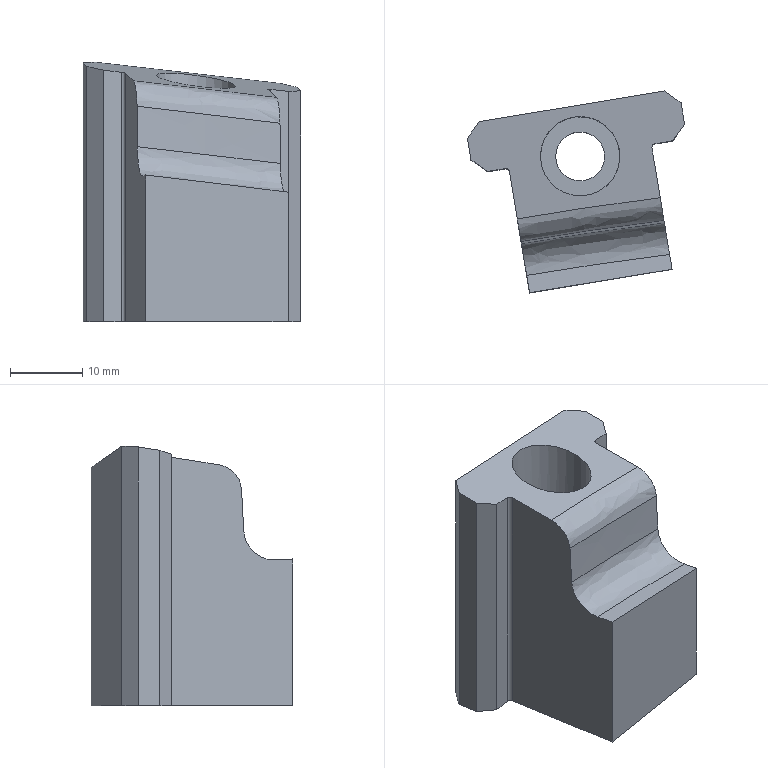Part | STEP file | gslz 2016.10.28-13_id510_x_t | 1 solid | 23 faces | box 30.087 x 27.932 x 35.938 mm | volume 13823 mm3 | plane 14 | spline 5 | cylinder 4 | commonest cylinder face diameters 1 x2 6.8 x1 11 x1